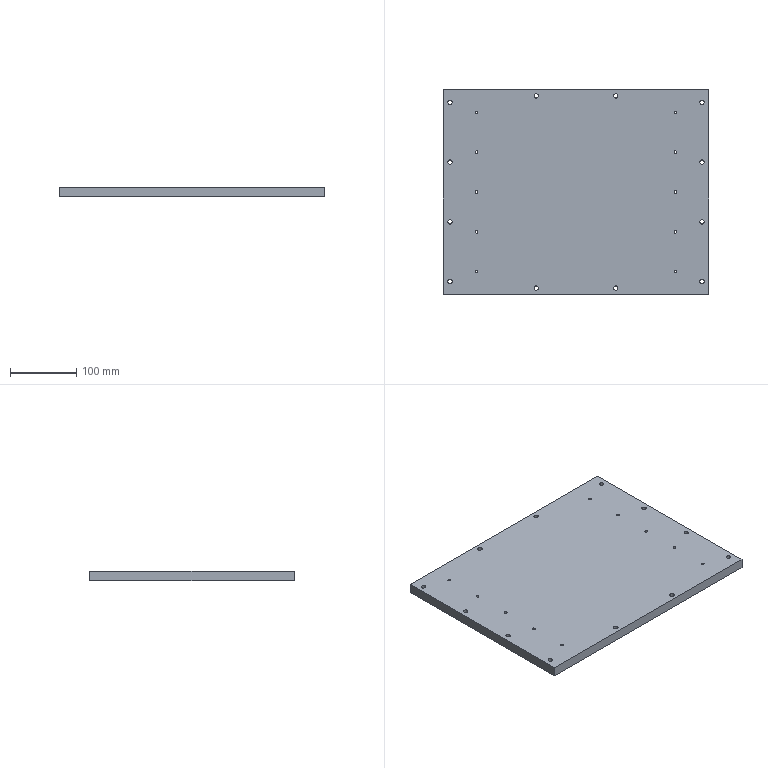Part | SolidWorks | features BaseBody 1 | 1 solid | 86 faces | box 400 x 308 x 15 mm | volume 1834801 mm3 | cylinder 68 | plane 18 | commonest cylinder face diameters 6.6 x24 11 x24 4.2 x20